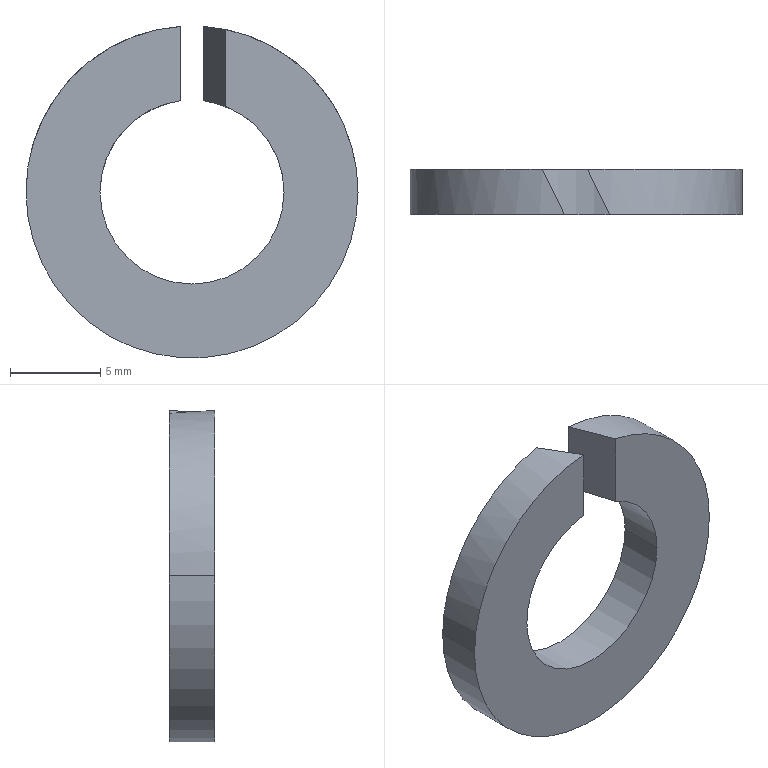Part | STEP file | ZZ24-M10-6 | 1 solid | 10 faces | box 18.4 x 2.5 x 18.378 mm | volume 434.673 mm3 | cylinder 6 | plane 4 | commonest cylinder face diameters 10.2 x3 18.4 x3
STEP:
#1=CARTESIAN_POINT('',(0.,0.,0.));
#2=DIRECTION('',(0.,0.,1.));
#3=DIRECTION('',(1.,0.,0.));
#4=AXIS2_PLACEMENT_3D('',#1,#2,#3);
#5=CARTESIAN_POINT('',(1.86,0.,4.749));
#6=VERTEX_POINT('',#5);
#7=CARTESIAN_POINT('',(0.6403,2.5,5.06));
#8=VERTEX_POINT('',#7);
#9=CARTESIAN_POINT('',(1.86,0.,4.749));
#10=CARTESIAN_POINT('',(1.467,0.8049,4.903));
#11=CARTESIAN_POINT('',(1.059,1.642,5.007));
#12=CARTESIAN_POINT('',(0.6403,2.5,5.06));
#13=(BOUNDED_CURVE()B_SPLINE_CURVE(3,(#9,#10,#11,#12),.UNSPECIFIED.,.F.,.F.)B_SPLINE_CURVE_WITH_KNOTS((4,4),(1.198,1.445),.PIECEWISE_BEZIER_KNOTS.)CURVE()GEOMETRIC_REPRESENTATION_ITEM()RATIONAL_B_SPLINE_CURVE((1.,0.9949,0.9949,1.))REPRESENTATION_ITEM(''));
#14=CARTESIAN_POINT('',(0.,2.5,0.));
#15=DIRECTION('',(0.,-1.,0.));
#16=DIRECTION('',(-1.,0.,0.001512));
#17=AXIS2_PLACEMENT_3D('',#14,#15,#16);
#18=CYLINDRICAL_SURFACE('',#17,5.1);
#19=CARTESIAN_POINT('',(4.341,2.5));
#20=CARTESIAN_POINT('',(4.344,2.464));
#21=CARTESIAN_POINT('',(4.352,2.391));
#22=CARTESIAN_POINT('',(4.363,2.281));
#23=CARTESIAN_POINT('',(4.374,2.17));
#24=CARTESIAN_POINT('',(4.386,2.059));
#25=CARTESIAN_POINT('',(4.397,1.948));
#26=CARTESIAN_POINT('',(4.408,1.836));
#27=CARTESIAN_POINT('',(4.419,1.723));
#28=CARTESIAN_POINT('',(4.431,1.61));
#29=CARTESIAN_POINT('',(4.442,1.497));
#30=CARTESIAN_POINT('',(4.453,1.384));
#31=CARTESIAN_POINT('',(4.464,1.27));
#32=CARTESIAN_POINT('',(4.476,1.156));
#33=CARTESIAN_POINT('',(4.487,1.041));
#34=CARTESIAN_POINT('',(4.498,0.9262));
#35=CARTESIAN_POINT('',(4.509,0.8111));
#36=CARTESIAN_POINT('',(4.521,0.6958));
#37=CARTESIAN_POINT('',(4.532,0.5802));
#38=CARTESIAN_POINT('',(4.543,0.4645));
#39=CARTESIAN_POINT('',(4.554,0.3486));
#40=CARTESIAN_POINT('',(4.566,0.2325));
#41=CARTESIAN_POINT('',(4.577,0.1163));
#42=CARTESIAN_POINT('',(4.584,0.03878));
#43=CARTESIAN_POINT('',(4.588,0.));
#44=B_SPLINE_CURVE_WITH_KNOTS('',3,(#19,#20,#21,#22,#23,#24,#25,#26,#27,#28,#29,#30,#31,#32,#33,#34,#35,#36,#37,#38,#39,#40,#41,#42,#43),.UNSPECIFIED.,.F.,.F.,(4,1,1,1,1,1,1,1,1,1,1,1,1,1,1,1,1,1,1,1,1,1,4),(1.198,1.209,1.22,1.231,1.243,1.254,1.265,1.276,1.287,1.299,1.31,1.321,1.332,1.344,1.355,1.366,1.377,1.389,1.4,1.411,1.422,1.434,1.445),.QUASI_UNIFORM_KNOTS.);
#45=(GEOMETRIC_REPRESENTATION_CONTEXT(2)PARAMETRIC_REPRESENTATION_CONTEXT()REPRESENTATION_CONTEXT('',''));
#46=DEFINITIONAL_REPRESENTATION('',(#44),#45);
#47=PCURVE('',#18,#46);
#48=CARTESIAN_POINT('',(1.86,0.,9.2));
#49=DIRECTION('',(-0.8988,-0.4384,0.));
#50=DIRECTION('',(0.4384,-0.8988,0.));
#51=AXIS2_PLACEMENT_3D('',#48,#49,#50);
#52=PLANE('',#51);
#53=CARTESIAN_POINT('',(0.,-4.451));
#54=CARTESIAN_POINT('',(-0.8955,-4.297));
#55=CARTESIAN_POINT('',(-1.827,-4.193));
#56=CARTESIAN_POINT('',(-2.782,-4.14));
#57=(BOUNDED_CURVE()B_SPLINE_CURVE(3,(#53,#54,#55,#56),.UNSPECIFIED.,.F.,.F.)B_SPLINE_CURVE_WITH_KNOTS((4,4),(1.198,1.445),.PIECEWISE_BEZIER_KNOTS.)CURVE()GEOMETRIC_REPRESENTATION_ITEM()RATIONAL_B_SPLINE_CURVE((1.,0.9949,0.9949,1.))REPRESENTATION_ITEM(''));
#58=(GEOMETRIC_REPRESENTATION_CONTEXT(2)PARAMETRIC_REPRESENTATION_CONTEXT()REPRESENTATION_CONTEXT('',''));
#59=DEFINITIONAL_REPRESENTATION('',(#57),#58);
#60=PCURVE('',#52,#59);
#61=SURFACE_CURVE('',#13,(#47,#60),.PCURVE_S1.);
#62=EDGE_CURVE('',#6,#8,#61,.T.);
#63=ORIENTED_EDGE('',*,*,#62,.F.);
#64=CARTESIAN_POINT('',(5.1,0.,-0.007712));
#65=VERTEX_POINT('',#64);
#66=CARTESIAN_POINT('',(0.,0.,0.));
#67=DIRECTION('',(0.,1.,0.));
#68=DIRECTION('',(1.,0.,-0.001512));
#69=AXIS2_PLACEMENT_3D('',#66,#67,#68);
#70=CIRCLE('',#69,5.1);
#71=CARTESIAN_POINT('',(9.425,2.5));
#72=DIRECTION('',(-1.,0.));
#73=VECTOR('',#72,1.);
#74=LINE('',#71,#73);
#75=(GEOMETRIC_REPRESENTATION_CONTEXT(2)PARAMETRIC_REPRESENTATION_CONTEXT()REPRESENTATION_CONTEXT('',''));
#76=DEFINITIONAL_REPRESENTATION('',(#74),#75);
#77=PCURVE('',#18,#76);
#78=CARTESIAN_POINT('',(0.,0.,0.));
#79=DIRECTION('',(0.,-1.,0.));
#80=DIRECTION('',(-1.,0.,0.001512));
#81=AXIS2_PLACEMENT_3D('',#78,#79,#80);
#82=PLANE('',#81);
#83=CARTESIAN_POINT('',(-5.1,0.));
#84=CARTESIAN_POINT('',(-5.1,8.833));
#85=CARTESIAN_POINT('',(2.55,4.417));
#86=CARTESIAN_POINT('',(10.2,0.));
#87=CARTESIAN_POINT('',(2.55,-4.417));
#88=CARTESIAN_POINT('',(-5.1,-8.833));
#89=CARTESIAN_POINT('',(-5.1,0.));
#90=(BOUNDED_CURVE()B_SPLINE_CURVE(2,(#83,#84,#85,#86,#87,#88,#89),.UNSPECIFIED.,.T.,.F.)B_SPLINE_CURVE_WITH_KNOTS((1,2,2,2,2,1),(-2.094,0.,2.094,4.189,6.283,8.378),.UNSPECIFIED.)CURVE()GEOMETRIC_REPRESENTATION_ITEM()RATIONAL_B_SPLINE_CURVE((1.,0.5,1.,0.5,1.,0.5,1.))REPRESENTATION_ITEM(''));
#91=(GEOMETRIC_REPRESENTATION_CONTEXT(2)PARAMETRIC_REPRESENTATION_CONTEXT()REPRESENTATION_CONTEXT('',''));
#92=DEFINITIONAL_REPRESENTATION('',(#90),#91);
#93=PCURVE('',#82,#92);
#94=SURFACE_CURVE('',#70,(#77,#93),.PCURVE_S1.);
#95=EDGE_CURVE('',#6,#65,#94,.T.);
#96=ORIENTED_EDGE('',*,*,#95,.T.);
#97=CARTESIAN_POINT('',(5.1,2.5,-0.007712));
#98=VERTEX_POINT('',#97);
#99=CARTESIAN_POINT('',(5.1,2.5,-0.007712));
#100=DIRECTION('',(0.,-1.,0.));
#101=VECTOR('',#100,1.);
#102=LINE('',#99,#101);
#103=CARTESIAN_POINT('',(3.142,0.));
#104=DIRECTION('',(0.,1.));
#105=VECTOR('',#104,1.);
#106=LINE('',#103,#105);
#107=(GEOMETRIC_REPRESENTATION_CONTEXT(2)PARAMETRIC_REPRESENTATION_CONTEXT()REPRESENTATION_CONTEXT('',''));
#108=DEFINITIONAL_REPRESENTATION('',(#106),#107);
#109=PCURVE('',#18,#108);
#110=CARTESIAN_POINT('',(0.,2.5,0.));
#111=DIRECTION('',(0.,-1.,0.));
#112=DIRECTION('',(-1.,0.,0.001512));
#113=AXIS2_PLACEMENT_3D('',#110,#111,#112);
#114=CYLINDRICAL_SURFACE('',#113,5.1);
#115=CARTESIAN_POINT('',(3.142,0.));
#116=DIRECTION('',(0.,1.));
#117=VECTOR('',#116,1.);
#118=LINE('',#115,#117);
#119=(GEOMETRIC_REPRESENTATION_CONTEXT(2)PARAMETRIC_REPRESENTATION_CONTEXT()REPRESENTATION_CONTEXT('',''));
#120=DEFINITIONAL_REPRESENTATION('',(#118),#119);
#121=PCURVE('',#114,#120);
#122=SURFACE_CURVE('',#102,(#109,#121),.PCURVE_S1.);
#123=EDGE_CURVE('',#98,#65,#122,.T.);
#124=ORIENTED_EDGE('',*,*,#123,.F.);
#125=CARTESIAN_POINT('',(0.,2.5,0.));
#126=DIRECTION('',(0.,-1.,0.));
#127=DIRECTION('',(-1.,0.,0.001512));
#128=AXIS2_PLACEMENT_3D('',#125,#126,#127);
#129=CIRCLE('',#128,5.1);
#130=CARTESIAN_POINT('',(0.,0.));
#131=DIRECTION('',(1.,0.));
#132=VECTOR('',#131,1.);
#133=LINE('',#130,#132);
#134=(GEOMETRIC_REPRESENTATION_CONTEXT(2)PARAMETRIC_REPRESENTATION_CONTEXT()REPRESENTATION_CONTEXT('',''));
#135=DEFINITIONAL_REPRESENTATION('',(#133),#134);
#136=PCURVE('',#18,#135);
#137=CARTESIAN_POINT('',(0.,2.5,0.));
#138=DIRECTION('',(0.,1.,0.));
#139=DIRECTION('',(1.,0.,-0.001512));
#140=AXIS2_PLACEMENT_3D('',#137,#138,#139);
#141=PLANE('',#140);
#142=CARTESIAN_POINT('',(-5.1,0.));
#143=CARTESIAN_POINT('',(-5.1,8.833));
#144=CARTESIAN_POINT('',(2.55,4.417));
#145=CARTESIAN_POINT('',(10.2,0.));
#146=CARTESIAN_POINT('',(2.55,-4.417));
#147=CARTESIAN_POINT('',(-5.1,-8.833));
#148=CARTESIAN_POINT('',(-5.1,0.));
#149=(BOUNDED_CURVE()B_SPLINE_CURVE(2,(#142,#143,#144,#145,#146,#147,#148),.UNSPECIFIED.,.T.,.F.)B_SPLINE_CURVE_WITH_KNOTS((1,2,2,2,2,1),(-2.094,0.,2.094,4.189,6.283,8.378),.UNSPECIFIED.)CURVE()GEOMETRIC_REPRESENTATION_ITEM()RATIONAL_B_SPLINE_CURVE((1.,0.5,1.,0.5,1.,0.5,1.))REPRESENTATION_ITEM(''));
#150=(GEOMETRIC_REPRESENTATION_CONTEXT(2)PARAMETRIC_REPRESENTATION_CONTEXT()REPRESENTATION_CONTEXT('',''));
#151=DEFINITIONAL_REPRESENTATION('',(#149),#150);
#152=PCURVE('',#141,#151);
#153=SURFACE_CURVE('',#129,(#136,#152),.PCURVE_S1.);
#154=EDGE_CURVE('',#98,#8,#153,.T.);
#155=ORIENTED_EDGE('',*,*,#154,.T.);
#156=EDGE_LOOP('',(#63,#96,#124,#155));
#157=FACE_BOUND('',#156,.F.);
#158=ADVANCED_FACE('',(#157),#18,.F.);
#159=CARTESIAN_POINT('',(-5.1,0.,0.007712));
#160=VERTEX_POINT('',#159);
#161=CARTESIAN_POINT('',(0.,0.,0.));
#162=DIRECTION('',(0.,1.,0.));
#163=DIRECTION('',(1.,0.,-0.001512));
#164=AXIS2_PLACEMENT_3D('',#161,#162,#163);
#165=CIRCLE('',#164,5.1);
#166=CARTESIAN_POINT('',(3.142,2.5));
#167=DIRECTION('',(-1.,0.));
#168=VECTOR('',#167,1.);
#169=LINE('',#166,#168);
#170=(GEOMETRIC_REPRESENTATION_CONTEXT(2)PARAMETRIC_REPRESENTATION_CONTEXT()REPRESENTATION_CONTEXT('',''));
#171=DEFINITIONAL_REPRESENTATION('',(#169),#170);
#172=PCURVE('',#114,#171);
#173=CARTESIAN_POINT('',(-5.1,0.));
#174=CARTESIAN_POINT('',(-5.1,8.833));
#175=CARTESIAN_POINT('',(2.55,4.417));
#176=CARTESIAN_POINT('',(10.2,0.));
#177=CARTESIAN_POINT('',(2.55,-4.417));
#178=CARTESIAN_POINT('',(-5.1,-8.833));
#179=CARTESIAN_POINT('',(-5.1,0.));
#180=(BOUNDED_CURVE()B_SPLINE_CURVE(2,(#173,#174,#175,#176,#177,#178,#179),.UNSPECIFIED.,.T.,.F.)B_SPLINE_CURVE_WITH_KNOTS((1,2,2,2,2,1),(-2.094,0.,2.094,4.189,6.283,8.378),.UNSPECIFIED.)CURVE()GEOMETRIC_REPRESENTATION_ITEM()RATIONAL_B_SPLINE_CURVE((1.,0.5,1.,0.5,1.,0.5,1.))REPRESENTATION_ITEM(''));
#181=(GEOMETRIC_REPRESENTATION_CONTEXT(2)PARAMETRIC_REPRESENTATION_CONTEXT()REPRESENTATION_CONTEXT('',''));
#182=DEFINITIONAL_REPRESENTATION('',(#180),#181);
#183=PCURVE('',#82,#182);
#184=SURFACE_CURVE('',#165,(#172,#183),.PCURVE_S1.);
#185=EDGE_CURVE('',#65,#160,#184,.T.);
#186=ORIENTED_EDGE('',*,*,#185,.T.);
#187=CARTESIAN_POINT('',(-5.1,2.5,0.007712));
#188=VERTEX_POINT('',#187);
#189=CARTESIAN_POINT('',(-5.1,2.5,0.007712));
#190=DIRECTION('',(0.,-1.,0.));
#191=VECTOR('',#190,1.);
#192=LINE('',#189,#191);
#193=CARTESIAN_POINT('',(0.,0.));
#194=DIRECTION('',(0.,1.));
#195=VECTOR('',#194,1.);
#196=LINE('',#193,#195);
#197=(GEOMETRIC_REPRESENTATION_CONTEXT(2)PARAMETRIC_REPRESENTATION_CONTEXT()REPRESENTATION_CONTEXT('',''));
#198=DEFINITIONAL_REPRESENTATION('',(#196),#197);
#199=PCURVE('',#114,#198);
#200=CARTESIAN_POINT('',(0.,2.5,0.));
#201=DIRECTION('',(0.,-1.,0.));
#202=DIRECTION('',(-1.,0.,0.001512));
#203=AXIS2_PLACEMENT_3D('',#200,#201,#202);
#204=CYLINDRICAL_SURFACE('',#203,5.1);
#205=CARTESIAN_POINT('',(6.283,0.));
#206=DIRECTION('',(0.,1.));
#207=VECTOR('',#206,1.);
#208=LINE('',#205,#207);
#209=(GEOMETRIC_REPRESENTATION_CONTEXT(2)PARAMETRIC_REPRESENTATION_CONTEXT()REPRESENTATION_CONTEXT('',''));
#210=DEFINITIONAL_REPRESENTATION('',(#208),#209);
#211=PCURVE('',#204,#210);
#212=SURFACE_CURVE('',#192,(#199,#211),.PCURVE_S1.);
#213=EDGE_CURVE('',#188,#160,#212,.T.);
#214=ORIENTED_EDGE('',*,*,#213,.F.);
#215=CARTESIAN_POINT('',(0.,2.5,0.));
#216=DIRECTION('',(0.,-1.,0.));
#217=DIRECTION('',(-1.,0.,0.001512));
#218=AXIS2_PLACEMENT_3D('',#215,#216,#217);
#219=CIRCLE('',#218,5.1);
#220=CARTESIAN_POINT('',(0.,0.));
#221=DIRECTION('',(1.,0.));
#222=VECTOR('',#221,1.);
#223=LINE('',#220,#222);
#224=(GEOMETRIC_REPRESENTATION_CONTEXT(2)PARAMETRIC_REPRESENTATION_CONTEXT()REPRESENTATION_CONTEXT('',''));
#225=DEFINITIONAL_REPRESENTATION('',(#223),#224);
#226=PCURVE('',#114,#225);
#227=CARTESIAN_POINT('',(-5.1,0.));
#228=CARTESIAN_POINT('',(-5.1,8.833));
#229=CARTESIAN_POINT('',(2.55,4.417));
#230=CARTESIAN_POINT('',(10.2,0.));
#231=CARTESIAN_POINT('',(2.55,-4.417));
#232=CARTESIAN_POINT('',(-5.1,-8.833));
#233=CARTESIAN_POINT('',(-5.1,0.));
#234=(BOUNDED_CURVE()B_SPLINE_CURVE(2,(#227,#228,#229,#230,#231,#232,#233),.UNSPECIFIED.,.T.,.F.)B_SPLINE_CURVE_WITH_KNOTS((1,2,2,2,2,1),(-2.094,0.,2.094,4.189,6.283,8.378),.UNSPECIFIED.)CURVE()GEOMETRIC_REPRESENTATION_ITEM()RATIONAL_B_SPLINE_CURVE((1.,0.5,1.,0.5,1.,0.5,1.))REPRESENTATION_ITEM(''));
#235=(GEOMETRIC_REPRESENTATION_CONTEXT(2)PARAMETRIC_REPRESENTATION_CONTEXT()REPRESENTATION_CONTEXT('',''));
#236=DEFINITIONAL_REPRESENTATION('',(#234),#235);
#237=PCURVE('',#141,#236);
#238=SURFACE_CURVE('',#219,(#226,#237),.PCURVE_S1.);
#239=EDGE_CURVE('',#188,#98,#238,.T.);
#240=ORIENTED_EDGE('',*,*,#239,.T.);
#241=ORIENTED_EDGE('',*,*,#123,.T.);
#242=EDGE_LOOP('',(#186,#214,#240,#241));
#243=FACE_BOUND('',#242,.F.);
#244=ADVANCED_FACE('',(#243),#114,.F.);
#245=CARTESIAN_POINT('',(-9.2,2.5,0.01391));
#246=VERTEX_POINT('',#245);
#247=CARTESIAN_POINT('',(9.2,2.5,-0.01391));
#248=VERTEX_POINT('',#247);
#249=CARTESIAN_POINT('',(0.,2.5,0.));
#250=DIRECTION('',(0.,-1.,0.));
#251=DIRECTION('',(-1.,0.,0.001512));
#252=AXIS2_PLACEMENT_3D('',#249,#250,#251);
#253=CIRCLE('',#252,9.2);
#254=CARTESIAN_POINT('',(0.,2.5,0.));
#255=DIRECTION('',(0.,-1.,0.));
#256=DIRECTION('',(-1.,0.,0.001512));
#257=AXIS2_PLACEMENT_3D('',#254,#255,#256);
#258=CYLINDRICAL_SURFACE('',#257,9.2);
#259=CARTESIAN_POINT('',(0.,0.));
#260=DIRECTION('',(1.,0.));
#261=VECTOR('',#260,1.);
#262=LINE('',#259,#261);
#263=(GEOMETRIC_REPRESENTATION_CONTEXT(2)PARAMETRIC_REPRESENTATION_CONTEXT()REPRESENTATION_CONTEXT('',''));
#264=DEFINITIONAL_REPRESENTATION('',(#262),#263);
#265=PCURVE('',#258,#264);
#266=CARTESIAN_POINT('',(-9.2,0.));
#267=CARTESIAN_POINT('',(-9.2,15.935));
#268=CARTESIAN_POINT('',(4.6,7.967));
#269=CARTESIAN_POINT('',(18.4,0.));
#270=CARTESIAN_POINT('',(4.6,-7.967));
#271=CARTESIAN_POINT('',(-9.2,-15.935));
#272=CARTESIAN_POINT('',(-9.2,0.));
#273=(BOUNDED_CURVE()B_SPLINE_CURVE(2,(#266,#267,#268,#269,#270,#271,#272),.UNSPECIFIED.,.T.,.F.)B_SPLINE_CURVE_WITH_KNOTS((1,2,2,2,2,1),(-2.094,0.,2.094,4.189,6.283,8.378),.UNSPECIFIED.)CURVE()GEOMETRIC_REPRESENTATION_ITEM()RATIONAL_B_SPLINE_CURVE((1.,0.5,1.,0.5,1.,0.5,1.))REPRESENTATION_ITEM(''));
#274=(GEOMETRIC_REPRESENTATION_CONTEXT(2)PARAMETRIC_REPRESENTATION_CONTEXT()REPRESENTATION_CONTEXT('',''));
#275=DEFINITIONAL_REPRESENTATION('',(#273),#274);
#276=PCURVE('',#141,#275);
#277=SURFACE_CURVE('',#253,(#265,#276),.PCURVE_S1.);
#278=EDGE_CURVE('',#246,#248,#277,.T.);
#279=ORIENTED_EDGE('',*,*,#278,.T.);
#280=CARTESIAN_POINT('',(9.2,0.,-0.01391));
#281=VERTEX_POINT('',#280);
#282=CARTESIAN_POINT('',(9.2,2.5,-0.01391));
#283=DIRECTION('',(0.,-1.,0.));
#284=VECTOR('',#283,1.);
#285=LINE('',#282,#284);
#286=CARTESIAN_POINT('',(3.142,0.));
#287=DIRECTION('',(0.,1.));
#288=VECTOR('',#287,1.);
#289=LINE('',#286,#288);
#290=(GEOMETRIC_REPRESENTATION_CONTEXT(2)PARAMETRIC_REPRESENTATION_CONTEXT()REPRESENTATION_CONTEXT('',''));
#291=DEFINITIONAL_REPRESENTATION('',(#289),#290);
#292=PCURVE('',#258,#291);
#293=CARTESIAN_POINT('',(0.,2.5,0.));
#294=DIRECTION('',(0.,-1.,0.));
#295=DIRECTION('',(-1.,0.,0.001512));
#296=AXIS2_PLACEMENT_3D('',#293,#294,#295);
#297=CYLINDRICAL_SURFACE('',#296,9.2);
#298=CARTESIAN_POINT('',(3.142,0.));
#299=DIRECTION('',(0.,1.));
#300=VECTOR('',#299,1.);
#301=LINE('',#298,#300);
#302=(GEOMETRIC_REPRESENTATION_CONTEXT(2)PARAMETRIC_REPRESENTATION_CONTEXT()REPRESENTATION_CONTEXT('',''));
#303=DEFINITIONAL_REPRESENTATION('',(#301),#302);
#304=PCURVE('',#297,#303);
#305=SURFACE_CURVE('',#285,(#292,#304),.PCURVE_S1.);
#306=EDGE_CURVE('',#248,#281,#305,.T.);
#307=ORIENTED_EDGE('',*,*,#306,.T.);
#308=CARTESIAN_POINT('',(-9.2,0.,0.01391));
#309=VERTEX_POINT('',#308);
#310=CARTESIAN_POINT('',(0.,0.,0.));
#311=DIRECTION('',(0.,1.,0.));
#312=DIRECTION('',(1.,0.,-0.001512));
#313=AXIS2_PLACEMENT_3D('',#310,#311,#312);
#314=CIRCLE('',#313,9.2);
#315=CARTESIAN_POINT('',(3.142,2.5));
#316=DIRECTION('',(-1.,0.));
#317=VECTOR('',#316,1.);
#318=LINE('',#315,#317);
#319=(GEOMETRIC_REPRESENTATION_CONTEXT(2)PARAMETRIC_REPRESENTATION_CONTEXT()REPRESENTATION_CONTEXT('',''));
#320=DEFINITIONAL_REPRESENTATION('',(#318),#319);
#321=PCURVE('',#258,#320);
#322=CARTESIAN_POINT('',(-9.2,0.));
#323=CARTESIAN_POINT('',(-9.2,15.935));
#324=CARTESIAN_POINT('',(4.6,7.967));
#325=CARTESIAN_POINT('',(18.4,0.));
#326=CARTESIAN_POINT('',(4.6,-7.967));
#327=CARTESIAN_POINT('',(-9.2,-15.935));
#328=CARTESIAN_POINT('',(-9.2,0.));
#329=(BOUNDED_CURVE()B_SPLINE_CURVE(2,(#322,#323,#324,#325,#326,#327,#328),.UNSPECIFIED.,.T.,.F.)B_SPLINE_CURVE_WITH_KNOTS((1,2,2,2,2,1),(-2.094,0.,2.094,4.189,6.283,8.378),.UNSPECIFIED.)CURVE()GEOMETRIC_REPRESENTATION_ITEM()RATIONAL_B_SPLINE_CURVE((1.,0.5,1.,0.5,1.,0.5,1.))REPRESENTATION_ITEM(''));
#330=(GEOMETRIC_REPRESENTATION_CONTEXT(2)PARAMETRIC_REPRESENTATION_CONTEXT()REPRESENTATION_CONTEXT('',''));
#331=DEFINITIONAL_REPRESENTATION('',(#329),#330);
#332=PCURVE('',#82,#331);
#333=SURFACE_CURVE('',#314,(#321,#332),.PCURVE_S1.);
#334=EDGE_CURVE('',#281,#309,#333,.T.);
#335=ORIENTED_EDGE('',*,*,#334,.T.);
#336=CARTESIAN_POINT('',(-9.2,2.5,0.01391));
#337=DIRECTION('',(0.,-1.,0.));
#338=VECTOR('',#337,1.);
#339=LINE('',#336,#338);
#340=CARTESIAN_POINT('',(0.,0.));
#341=DIRECTION('',(0.,1.));
#342=VECTOR('',#341,1.);
#343=LINE('',#340,#342);
#344=(GEOMETRIC_REPRESENTATION_CONTEXT(2)PARAMETRIC_REPRESENTATION_CONTEXT()REPRESENTATION_CONTEXT('',''));
#345=DEFINITIONAL_REPRESENTATION('',(#343),#344);
#346=PCURVE('',#258,#345);
#347=CARTESIAN_POINT('',(0.,2.5,0.));
#348=DIRECTION('',(0.,-1.,0.));
#349=DIRECTION('',(-1.,0.,0.001512));
#350=AXIS2_PLACEMENT_3D('',#347,#348,#349);
#351=CYLINDRICAL_SURFACE('',#350,9.2);
#352=CARTESIAN_POINT('',(6.283,0.));
#353=DIRECTION('',(0.,1.));
#354=VECTOR('',#353,1.);
#355=LINE('',#352,#354);
#356=(GEOMETRIC_REPRESENTATION_CONTEXT(2)PARAMETRIC_REPRESENTATION_CONTEXT()REPRESENTATION_CONTEXT('',''));
#357=DEFINITIONAL_REPRESENTATION('',(#355),#356);
#358=PCURVE('',#351,#357);
#359=SURFACE_CURVE('',#339,(#346,#358),.PCURVE_S1.);
#360=EDGE_CURVE('',#246,#309,#359,.T.);
#361=ORIENTED_EDGE('',*,*,#360,.F.);
#362=EDGE_LOOP('',(#279,#307,#335,#361));
#363=FACE_BOUND('',#362,.T.);
#364=ADVANCED_FACE('',(#363),#258,.T.);
#365=CARTESIAN_POINT('',(-1.86,2.5,9.01));
#366=VERTEX_POINT('',#365);
#367=CARTESIAN_POINT('',(0.,2.5,0.));
#368=DIRECTION('',(0.,-1.,0.));
#369=DIRECTION('',(-1.,0.,0.001512));
#370=AXIS2_PLACEMENT_3D('',#367,#368,#369);
#371=CIRCLE('',#370,9.2);
#372=CARTESIAN_POINT('',(0.,0.));
#373=DIRECTION('',(1.,0.));
#374=VECTOR('',#373,1.);
#375=LINE('',#372,#374);
#376=(GEOMETRIC_REPRESENTATION_CONTEXT(2)PARAMETRIC_REPRESENTATION_CONTEXT()REPRESENTATION_CONTEXT('',''));
#377=DEFINITIONAL_REPRESENTATION('',(#375),#376);
#378=PCURVE('',#351,#377);
#379=CARTESIAN_POINT('',(-9.2,0.));
#380=CARTESIAN_POINT('',(-9.2,15.935));
#381=CARTESIAN_POINT('',(4.6,7.967));
#382=CARTESIAN_POINT('',(18.4,0.));
#383=CARTESIAN_POINT('',(4.6,-7.967));
#384=CARTESIAN_POINT('',(-9.2,-15.935));
#385=CARTESIAN_POINT('',(-9.2,0.));
#386=(BOUNDED_CURVE()B_SPLINE_CURVE(2,(#379,#380,#381,#382,#383,#384,#385),.UNSPECIFIED.,.T.,.F.)B_SPLINE_CURVE_WITH_KNOTS((1,2,2,2,2,1),(-2.094,0.,2.094,4.189,6.283,8.378),.UNSPECIFIED.)CURVE()GEOMETRIC_REPRESENTATION_ITEM()RATIONAL_B_SPLINE_CURVE((1.,0.5,1.,0.5,1.,0.5,1.))REPRESENTATION_ITEM(''));
#387=(GEOMETRIC_REPRESENTATION_CONTEXT(2)PARAMETRIC_REPRESENTATION_CONTEXT()REPRESENTATION_CONTEXT('',''));
#388=DEFINITIONAL_REPRESENTATION('',(#386),#387);
#389=PCURVE('',#141,#388);
#390=SURFACE_CURVE('',#371,(#378,#389),.PCURVE_S1.);
#391=EDGE_CURVE('',#366,#246,#390,.T.);
#392=ORIENTED_EDGE('',*,*,#391,.T.);
#393=ORIENTED_EDGE('',*,*,#360,.T.);
#394=CARTESIAN_POINT('',(-0.6403,0.,9.178));
#395=VERTEX_POINT('',#394);
#396=CARTESIAN_POINT('',(0.,0.,0.));
#397=DIRECTION('',(0.,1.,0.));
#398=DIRECTION('',(1.,0.,-0.001512));
#399=AXIS2_PLACEMENT_3D('',#396,#397,#398);
#400=CIRCLE('',#399,9.2);
#401=CARTESIAN_POINT('',(9.425,2.5));
#402=DIRECTION('',(-1.,0.));
#403=VECTOR('',#402,1.);
#404=LINE('',#401,#403);
#405=(GEOMETRIC_REPRESENTATION_CONTEXT(2)PARAMETRIC_REPRESENTATION_CONTEXT()REPRESENTATION_CONTEXT('',''));
#406=DEFINITIONAL_REPRESENTATION('',(#404),#405);
#407=PCURVE('',#351,#406);
#408=CARTESIAN_POINT('',(-9.2,0.));
#409=CARTESIAN_POINT('',(-9.2,15.935));
#410=CARTESIAN_POINT('',(4.6,7.967));
#411=CARTESIAN_POINT('',(18.4,0.));
#412=CARTESIAN_POINT('',(4.6,-7.967));
#413=CARTESIAN_POINT('',(-9.2,-15.935));
#414=CARTESIAN_POINT('',(-9.2,0.));
#415=(BOUNDED_CURVE()B_SPLINE_CURVE(2,(#408,#409,#410,#411,#412,#413,#414),.UNSPECIFIED.,.T.,.F.)B_SPLINE_CURVE_WITH_KNOTS((1,2,2,2,2,1),(-2.094,0.,2.094,4.189,6.283,8.378),.UNSPECIFIED.)CURVE()GEOMETRIC_REPRESENTATION_ITEM()RATIONAL_B_SPLINE_CURVE((1.,0.5,1.,0.5,1.,0.5,1.))REPRESENTATION_ITEM(''));
#416=(GEOMETRIC_REPRESENTATION_CONTEXT(2)PARAMETRIC_REPRESENTATION_CONTEXT()REPRESENTATION_CONTEXT('',''));
#417=DEFINITIONAL_REPRESENTATION('',(#415),#416);
#418=PCURVE('',#82,#417);
#419=SURFACE_CURVE('',#400,(#407,#418),.PCURVE_S1.);
#420=EDGE_CURVE('',#309,#395,#419,.T.);
#421=ORIENTED_EDGE('',*,*,#420,.T.);
#422=CARTESIAN_POINT('',(-0.6403,0.,9.178));
#423=CARTESIAN_POINT('',(-1.05,0.8404,9.149));
#424=CARTESIAN_POINT('',(-1.457,1.675,9.093));
#425=CARTESIAN_POINT('',(-1.86,2.5,9.01));
#426=(BOUNDED_CURVE()B_SPLINE_CURVE(3,(#422,#423,#424,#425),.UNSPECIFIED.,.F.,.F.)B_SPLINE_CURVE_WITH_KNOTS((4,4),(1.64,1.774),.PIECEWISE_BEZIER_KNOTS.)CURVE()GEOMETRIC_REPRESENTATION_ITEM()RATIONAL_B_SPLINE_CURVE((1.,0.9985,0.9985,1.))REPRESENTATION_ITEM(''));
#427=CARTESIAN_POINT('',(4.784,2.5));
#428=CARTESIAN_POINT('',(4.786,2.462));
#429=CARTESIAN_POINT('',(4.79,2.386));
#430=CARTESIAN_POINT('',(4.796,2.271));
#431=CARTESIAN_POINT('',(4.802,2.157));
#432=CARTESIAN_POINT('',(4.808,2.043));
#433=CARTESIAN_POINT('',(4.814,1.928));
#434=CARTESIAN_POINT('',(4.82,1.814));
#435=CARTESIAN_POINT('',(4.826,1.7));
#436=CARTESIAN_POINT('',(4.832,1.586));
#437=CARTESIAN_POINT('',(4.838,1.472));
#438=CARTESIAN_POINT('',(4.844,1.358));
#439=CARTESIAN_POINT('',(4.851,1.244));
#440=CARTESIAN_POINT('',(4.857,1.131));
#441=CARTESIAN_POINT('',(4.863,1.017));
#442=CARTESIAN_POINT('',(4.869,0.9034));
#443=CARTESIAN_POINT('',(4.875,0.79));
#444=CARTESIAN_POINT('',(4.881,0.6767));
#445=CARTESIAN_POINT('',(4.887,0.5636));
#446=CARTESIAN_POINT('',(4.893,0.4506));
#447=CARTESIAN_POINT('',(4.899,0.3377));
#448=CARTESIAN_POINT('',(4.905,0.225));
#449=CARTESIAN_POINT('',(4.911,0.1124));
#450=CARTESIAN_POINT('',(4.915,0.03745));
#451=CARTESIAN_POINT('',(4.917,0.));
#452=B_SPLINE_CURVE_WITH_KNOTS('',3,(#427,#428,#429,#430,#431,#432,#433,#434,#435,#436,#437,#438,#439,#440,#441,#442,#443,#444,#445,#446,#447,#448,#449,#450,#451),.UNSPECIFIED.,.F.,.F.,(4,1,1,1,1,1,1,1,1,1,1,1,1,1,1,1,1,1,1,1,1,1,4),(1.64,1.647,1.653,1.659,1.665,1.671,1.677,1.683,1.689,1.695,1.701,1.707,1.713,1.72,1.726,1.732,1.738,1.744,1.75,1.756,1.762,1.768,1.774),.QUASI_UNIFORM_KNOTS.);
#453=(GEOMETRIC_REPRESENTATION_CONTEXT(2)PARAMETRIC_REPRESENTATION_CONTEXT()REPRESENTATION_CONTEXT('',''));
#454=DEFINITIONAL_REPRESENTATION('',(#452),#453);
#455=PCURVE('',#351,#454);
#456=CARTESIAN_POINT('',(-1.86,2.5,9.2));
#457=DIRECTION('',(0.8988,0.4384,0.));
#458=DIRECTION('',(-0.4384,0.8988,0.));
#459=AXIS2_PLACEMENT_3D('',#456,#457,#458);
#460=PLANE('',#459);
#461=CARTESIAN_POINT('',(-2.782,-0.02231));
#462=CARTESIAN_POINT('',(-1.846,-0.05091));
#463=CARTESIAN_POINT('',(-0.9179,-0.1069));
#464=CARTESIAN_POINT('',(0.,-0.1899));
#465=(BOUNDED_CURVE()B_SPLINE_CURVE(3,(#461,#462,#463,#464),.UNSPECIFIED.,.F.,.F.)B_SPLINE_CURVE_WITH_KNOTS((4,4),(1.64,1.774),.PIECEWISE_BEZIER_KNOTS.)CURVE()GEOMETRIC_REPRESENTATION_ITEM()RATIONAL_B_SPLINE_CURVE((1.,0.9985,0.9985,1.))REPRESENTATION_ITEM(''));
#466=(GEOMETRIC_REPRESENTATION_CONTEXT(2)PARAMETRIC_REPRESENTATION_CONTEXT()REPRESENTATION_CONTEXT('',''));
#467=DEFINITIONAL_REPRESENTATION('',(#465),#466);
#468=PCURVE('',#460,#467);
#469=SURFACE_CURVE('',#426,(#455,#468),.PCURVE_S1.);
#470=EDGE_CURVE('',#395,#366,#469,.T.);
#471=ORIENTED_EDGE('',*,*,#470,.T.);
#472=EDGE_LOOP('',(#392,#393,#421,#471));
#473=FACE_BOUND('',#472,.T.);
#474=ADVANCED_FACE('',(#473),#351,.T.);
#475=CARTESIAN_POINT('',(-0.6403,0.,5.06));
#476=VERTEX_POINT('',#475);
#477=CARTESIAN_POINT('',(-0.6403,0.,9.2));
#478=DIRECTION('',(0.,0.,-1.));
#479=VECTOR('',#478,1.);
#480=LINE('',#477,#479);
#481=CARTESIAN_POINT('',(0.6542,-9.199));
#482=DIRECTION('',(-0.001512,1.));
#483=VECTOR('',#482,1.);
#484=LINE('',#481,#483);
#485=(GEOMETRIC_REPRESENTATION_CONTEXT(2)PARAMETRIC_REPRESENTATION_CONTEXT()REPRESENTATION_CONTEXT('',''));
#486=DEFINITIONAL_REPRESENTATION('',(#484),#485);
#487=PCURVE('',#82,#486);
#488=CARTESIAN_POINT('',(-2.782,0.));
#489=DIRECTION('',(0.,-1.));
#490=VECTOR('',#489,1.);
#491=LINE('',#488,#490);
#492=(GEOMETRIC_REPRESENTATION_CONTEXT(2)PARAMETRIC_REPRESENTATION_CONTEXT()REPRESENTATION_CONTEXT('',''));
#493=DEFINITIONAL_REPRESENTATION('',(#491),#492);
#494=PCURVE('',#460,#493);
#495=SURFACE_CURVE('',#480,(#487,#494),.PCURVE_S1.);
#496=EDGE_CURVE('',#395,#476,#495,.T.);
#497=ORIENTED_EDGE('',*,*,#496,.F.);
#498=ORIENTED_EDGE('',*,*,#420,.F.);
#499=ORIENTED_EDGE('',*,*,#334,.F.);
#500=CARTESIAN_POINT('',(1.86,0.,9.01));
#501=VERTEX_POINT('',#500);
#502=CARTESIAN_POINT('',(0.,0.,0.));
#503=DIRECTION('',(0.,1.,0.));
#504=DIRECTION('',(1.,0.,-0.001512));
#505=AXIS2_PLACEMENT_3D('',#502,#503,#504);
#506=CIRCLE('',#505,9.2);
#507=CARTESIAN_POINT('',(-9.2,0.));
#508=CARTESIAN_POINT('',(-9.2,15.935));
#509=CARTESIAN_POINT('',(4.6,7.967));
#510=CARTESIAN_POINT('',(18.4,0.));
#511=CARTESIAN_POINT('',(4.6,-7.967));
#512=CARTESIAN_POINT('',(-9.2,-15.935));
#513=CARTESIAN_POINT('',(-9.2,0.));
#514=(BOUNDED_CURVE()B_SPLINE_CURVE(2,(#507,#508,#509,#510,#511,#512,#513),.UNSPECIFIED.,.T.,.F.)B_SPLINE_CURVE_WITH_KNOTS((1,2,2,2,2,1),(-2.094,0.,2.094,4.189,6.283,8.378),.UNSPECIFIED.)CURVE()GEOMETRIC_REPRESENTATION_ITEM()RATIONAL_B_SPLINE_CURVE((1.,0.5,1.,0.5,1.,0.5,1.))REPRESENTATION_ITEM(''));
#515=(GEOMETRIC_REPRESENTATION_CONTEXT(2)PARAMETRIC_REPRESENTATION_CONTEXT()REPRESENTATION_CONTEXT('',''));
#516=DEFINITIONAL_REPRESENTATION('',(#514),#515);
#517=PCURVE('',#82,#516);
#518=CARTESIAN_POINT('',(9.425,2.5));
#519=DIRECTION('',(-1.,0.));
#520=VECTOR('',#519,1.);
#521=LINE('',#518,#520);
#522=(GEOMETRIC_REPRESENTATION_CONTEXT(2)PARAMETRIC_REPRESENTATION_CONTEXT()REPRESENTATION_CONTEXT('',''));
#523=DEFINITIONAL_REPRESENTATION('',(#521),#522);
#524=PCURVE('',#297,#523);
#525=SURFACE_CURVE('',#506,(#517,#524),.PCURVE_S1.);
#526=EDGE_CURVE('',#501,#281,#525,.T.);
#527=ORIENTED_EDGE('',*,*,#526,.F.);
#528=CARTESIAN_POINT('',(1.86,0.,9.2));
#529=DIRECTION('',(0.,0.,-1.));
#530=VECTOR('',#529,1.);
#531=LINE('',#528,#530);
#532=CARTESIAN_POINT('',(-1.846,-9.203));
#533=DIRECTION('',(-0.001512,1.));
#534=VECTOR('',#533,1.);
#535=LINE('',#532,#534);
#536=(GEOMETRIC_REPRESENTATION_CONTEXT(2)PARAMETRIC_REPRESENTATION_CONTEXT()REPRESENTATION_CONTEXT('',''));
#537=DEFINITIONAL_REPRESENTATION('',(#535),#536);
#538=PCURVE('',#82,#537);
#539=CARTESIAN_POINT('',(0.,0.));
#540=DIRECTION('',(0.,-1.));
#541=VECTOR('',#540,1.);
#542=LINE('',#539,#541);
#543=(GEOMETRIC_REPRESENTATION_CONTEXT(2)PARAMETRIC_REPRESENTATION_CONTEXT()REPRESENTATION_CONTEXT('',''));
#544=DEFINITIONAL_REPRESENTATION('',(#542),#543);
#545=PCURVE('',#52,#544);
#546=SURFACE_CURVE('',#531,(#538,#545),.PCURVE_S1.);
#547=EDGE_CURVE('',#501,#6,#546,.T.);
#548=ORIENTED_EDGE('',*,*,#547,.T.);
#549=ORIENTED_EDGE('',*,*,#95,.T.);
#550=ORIENTED_EDGE('',*,*,#185,.T.);
#551=CARTESIAN_POINT('',(0.,0.,0.));
#552=DIRECTION('',(0.,1.,0.));
#553=DIRECTION('',(1.,0.,-0.001512));
#554=AXIS2_PLACEMENT_3D('',#551,#552,#553);
#555=CIRCLE('',#554,5.1);
#556=CARTESIAN_POINT('',(-5.1,0.));
#557=CARTESIAN_POINT('',(-5.1,8.833));
#558=CARTESIAN_POINT('',(2.55,4.417));
#559=CARTESIAN_POINT('',(10.2,0.));
#560=CARTESIAN_POINT('',(2.55,-4.417));
#561=CARTESIAN_POINT('',(-5.1,-8.833));
#562=CARTESIAN_POINT('',(-5.1,0.));
#563=(BOUNDED_CURVE()B_SPLINE_CURVE(2,(#556,#557,#558,#559,#560,#561,#562),.UNSPECIFIED.,.T.,.F.)B_SPLINE_CURVE_WITH_KNOTS((1,2,2,2,2,1),(-2.094,0.,2.094,4.189,6.283,8.378),.UNSPECIFIED.)CURVE()GEOMETRIC_REPRESENTATION_ITEM()RATIONAL_B_SPLINE_CURVE((1.,0.5,1.,0.5,1.,0.5,1.))REPRESENTATION_ITEM(''));
#564=(GEOMETRIC_REPRESENTATION_CONTEXT(2)PARAMETRIC_REPRESENTATION_CONTEXT()REPRESENTATION_CONTEXT('',''));
#565=DEFINITIONAL_REPRESENTATION('',(#563),#564);
#566=PCURVE('',#82,#565);
#567=CARTESIAN_POINT('',(9.425,2.5));
#568=DIRECTION('',(-1.,0.));
#569=VECTOR('',#568,1.);
#570=LINE('',#567,#569);
#571=(GEOMETRIC_REPRESENTATION_CONTEXT(2)PARAMETRIC_REPRESENTATION_CONTEXT()REPRESENTATION_CONTEXT('',''));
#572=DEFINITIONAL_REPRESENTATION('',(#570),#571);
#573=PCURVE('',#204,#572);
#574=SURFACE_CURVE('',#555,(#566,#573),.PCURVE_S1.);
#575=EDGE_CURVE('',#160,#476,#574,.T.);
#576=ORIENTED_EDGE('',*,*,#575,.T.);
#577=EDGE_LOOP('',(#497,#498,#499,#527,#548,#549,#550,#576));
#578=FACE_BOUND('',#577,.T.);
#579=ADVANCED_FACE('',(#578),#82,.T.);
#580=CARTESIAN_POINT('',(0.6403,2.5,9.178));
#581=VERTEX_POINT('',#580);
#582=CARTESIAN_POINT('',(0.6403,2.5,9.2));
#583=DIRECTION('',(0.,0.,-1.));
#584=VECTOR('',#583,1.);
#585=LINE('',#582,#584);
#586=CARTESIAN_POINT('',(0.6264,-9.201));
#587=DIRECTION('',(0.001512,1.));
#588=VECTOR('',#587,1.);
#589=LINE('',#586,#588);
#590=(GEOMETRIC_REPRESENTATION_CONTEXT(2)PARAMETRIC_REPRESENTATION_CONTEXT()REPRESENTATION_CONTEXT('',''));
#591=DEFINITIONAL_REPRESENTATION('',(#589),#590);
#592=PCURVE('',#141,#591);
#593=CARTESIAN_POINT('',(-2.782,0.));
#594=DIRECTION('',(0.,-1.));
#595=VECTOR('',#594,1.);
#596=LINE('',#593,#595);
#597=(GEOMETRIC_REPRESENTATION_CONTEXT(2)PARAMETRIC_REPRESENTATION_CONTEXT()REPRESENTATION_CONTEXT('',''));
#598=DEFINITIONAL_REPRESENTATION('',(#596),#597);
#599=PCURVE('',#52,#598);
#600=SURFACE_CURVE('',#585,(#592,#599),.PCURVE_S1.);
#601=EDGE_CURVE('',#581,#8,#600,.T.);
#602=ORIENTED_EDGE('',*,*,#601,.F.);
#603=CARTESIAN_POINT('',(0.,2.5,0.));
#604=DIRECTION('',(0.,-1.,0.));
#605=DIRECTION('',(-1.,0.,0.001512));
#606=AXIS2_PLACEMENT_3D('',#603,#604,#605);
#607=CIRCLE('',#606,9.2);
#608=CARTESIAN_POINT('',(-9.2,0.));
#609=CARTESIAN_POINT('',(-9.2,15.935));
#610=CARTESIAN_POINT('',(4.6,7.967));
#611=CARTESIAN_POINT('',(18.4,0.));
#612=CARTESIAN_POINT('',(4.6,-7.967));
#613=CARTESIAN_POINT('',(-9.2,-15.935));
#614=CARTESIAN_POINT('',(-9.2,0.));
#615=(BOUNDED_CURVE()B_SPLINE_CURVE(2,(#608,#609,#610,#611,#612,#613,#614),.UNSPECIFIED.,.T.,.F.)B_SPLINE_CURVE_WITH_KNOTS((1,2,2,2,2,1),(-2.094,0.,2.094,4.189,6.283,8.378),.UNSPECIFIED.)CURVE()GEOMETRIC_REPRESENTATION_ITEM()RATIONAL_B_SPLINE_CURVE((1.,0.5,1.,0.5,1.,0.5,1.))REPRESENTATION_ITEM(''));
#616=(GEOMETRIC_REPRESENTATION_CONTEXT(2)PARAMETRIC_REPRESENTATION_CONTEXT()REPRESENTATION_CONTEXT('',''));
#617=DEFINITIONAL_REPRESENTATION('',(#615),#616);
#618=PCURVE('',#141,#617);
#619=CARTESIAN_POINT('',(0.,0.));
#620=DIRECTION('',(1.,0.));
#621=VECTOR('',#620,1.);
#622=LINE('',#619,#621);
#623=(GEOMETRIC_REPRESENTATION_CONTEXT(2)PARAMETRIC_REPRESENTATION_CONTEXT()REPRESENTATION_CONTEXT('',''));
#624=DEFINITIONAL_REPRESENTATION('',(#622),#623);
#625=PCURVE('',#297,#624);
#626=SURFACE_CURVE('',#607,(#618,#625),.PCURVE_S1.);
#627=EDGE_CURVE('',#248,#581,#626,.T.);
#628=ORIENTED_EDGE('',*,*,#627,.F.);
#629=ORIENTED_EDGE('',*,*,#278,.F.);
#630=ORIENTED_EDGE('',*,*,#391,.F.);
#631=CARTESIAN_POINT('',(-1.86,2.5,4.749));
#632=VERTEX_POINT('',#631);
#633=CARTESIAN_POINT('',(-1.86,2.5,9.2));
#634=DIRECTION('',(0.,0.,-1.));
#635=VECTOR('',#634,1.);
#636=LINE('',#633,#635);
#637=CARTESIAN_POINT('',(-1.874,-9.197));
#638=DIRECTION('',(0.001512,1.));
#639=VECTOR('',#638,1.);
#640=LINE('',#637,#639);
#641=(GEOMETRIC_REPRESENTATION_CONTEXT(2)PARAMETRIC_REPRESENTATION_CONTEXT()REPRESENTATION_CONTEXT('',''));
#642=DEFINITIONAL_REPRESENTATION('',(#640),#641);
#643=PCURVE('',#141,#642);
#644=CARTESIAN_POINT('',(0.,0.));
#645=DIRECTION('',(0.,-1.));
#646=VECTOR('',#645,1.);
#647=LINE('',#644,#646);
#648=(GEOMETRIC_REPRESENTATION_CONTEXT(2)PARAMETRIC_REPRESENTATION_CONTEXT()REPRESENTATION_CONTEXT('',''));
#649=DEFINITIONAL_REPRESENTATION('',(#647),#648);
#650=PCURVE('',#460,#649);
#651=SURFACE_CURVE('',#636,(#643,#650),.PCURVE_S1.);
#652=EDGE_CURVE('',#366,#632,#651,.T.);
#653=ORIENTED_EDGE('',*,*,#652,.T.);
#654=CARTESIAN_POINT('',(0.,2.5,0.));
#655=DIRECTION('',(0.,-1.,0.));
#656=DIRECTION('',(-1.,0.,0.001512));
#657=AXIS2_PLACEMENT_3D('',#654,#655,#656);
#658=CIRCLE('',#657,5.1);
#659=CARTESIAN_POINT('',(-5.1,0.));
#660=CARTESIAN_POINT('',(-5.1,8.833));
#661=CARTESIAN_POINT('',(2.55,4.417));
#662=CARTESIAN_POINT('',(10.2,0.));
#663=CARTESIAN_POINT('',(2.55,-4.417));
#664=CARTESIAN_POINT('',(-5.1,-8.833));
#665=CARTESIAN_POINT('',(-5.1,0.));
#666=(BOUNDED_CURVE()B_SPLINE_CURVE(2,(#659,#660,#661,#662,#663,#664,#665),.UNSPECIFIED.,.T.,.F.)B_SPLINE_CURVE_WITH_KNOTS((1,2,2,2,2,1),(-2.094,0.,2.094,4.189,6.283,8.378),.UNSPECIFIED.)CURVE()GEOMETRIC_REPRESENTATION_ITEM()RATIONAL_B_SPLINE_CURVE((1.,0.5,1.,0.5,1.,0.5,1.))REPRESENTATION_ITEM(''));
#667=(GEOMETRIC_REPRESENTATION_CONTEXT(2)PARAMETRIC_REPRESENTATION_CONTEXT()REPRESENTATION_CONTEXT('',''));
#668=DEFINITIONAL_REPRESENTATION('',(#666),#667);
#669=PCURVE('',#141,#668);
#670=CARTESIAN_POINT('',(0.,0.));
#671=DIRECTION('',(1.,0.));
#672=VECTOR('',#671,1.);
#673=LINE('',#670,#672);
#674=(GEOMETRIC_REPRESENTATION_CONTEXT(2)PARAMETRIC_REPRESENTATION_CONTEXT()REPRESENTATION_CONTEXT('',''));
#675=DEFINITIONAL_REPRESENTATION('',(#673),#674);
#676=PCURVE('',#204,#675);
#677=SURFACE_CURVE('',#658,(#669,#676),.PCURVE_S1.);
#678=EDGE_CURVE('',#632,#188,#677,.T.);
#679=ORIENTED_EDGE('',*,*,#678,.T.);
#680=ORIENTED_EDGE('',*,*,#239,.T.);
#681=ORIENTED_EDGE('',*,*,#154,.T.);
#682=EDGE_LOOP('',(#602,#628,#629,#630,#653,#679,#680,#681));
#683=FACE_BOUND('',#682,.T.);
#684=ADVANCED_FACE('',(#683),#141,.T.);
#685=ORIENTED_EDGE('',*,*,#306,.F.);
#686=ORIENTED_EDGE('',*,*,#627,.T.);
#687=CARTESIAN_POINT('',(0.6403,2.5,9.178));
#688=CARTESIAN_POINT('',(1.05,1.66,9.149));
#689=CARTESIAN_POINT('',(1.457,0.825,9.093));
#690=CARTESIAN_POINT('',(1.86,0.,9.01));
#691=(BOUNDED_CURVE()B_SPLINE_CURVE(3,(#687,#688,#689,#690),.UNSPECIFIED.,.F.,.F.)B_SPLINE_CURVE_WITH_KNOTS((4,4),(4.782,4.916),.PIECEWISE_BEZIER_KNOTS.)CURVE()GEOMETRIC_REPRESENTATION_ITEM()RATIONAL_B_SPLINE_CURVE((1.,0.9985,0.9985,1.))REPRESENTATION_ITEM(''));
#692=CARTESIAN_POINT('',(4.644,0.));
#693=CARTESIAN_POINT('',(4.642,0.03814));
#694=CARTESIAN_POINT('',(4.638,0.1144));
#695=CARTESIAN_POINT('',(4.632,0.2288));
#696=CARTESIAN_POINT('',(4.626,0.3431));
#697=CARTESIAN_POINT('',(4.62,0.4574));
#698=CARTESIAN_POINT('',(4.614,0.5717));
#699=CARTESIAN_POINT('',(4.608,0.6859));
#700=CARTESIAN_POINT('',(4.602,0.8));
#701=CARTESIAN_POINT('',(4.596,0.9141));
#702=CARTESIAN_POINT('',(4.589,1.028));
#703=CARTESIAN_POINT('',(4.583,1.142));
#704=CARTESIAN_POINT('',(4.577,1.256));
#705=CARTESIAN_POINT('',(4.571,1.369));
#706=CARTESIAN_POINT('',(4.565,1.483));
#707=CARTESIAN_POINT('',(4.559,1.597));
#708=CARTESIAN_POINT('',(4.553,1.71));
#709=CARTESIAN_POINT('',(4.547,1.823));
#710=CARTESIAN_POINT('',(4.541,1.936));
#711=CARTESIAN_POINT('',(4.535,2.049));
#712=CARTESIAN_POINT('',(4.529,2.162));
#713=CARTESIAN_POINT('',(4.523,2.275));
#714=CARTESIAN_POINT('',(4.516,2.388));
#715=CARTESIAN_POINT('',(4.512,2.463));
#716=CARTESIAN_POINT('',(4.51,2.5));
#717=B_SPLINE_CURVE_WITH_KNOTS('',3,(#692,#693,#694,#695,#696,#697,#698,#699,#700,#701,#702,#703,#704,#705,#706,#707,#708,#709,#710,#711,#712,#713,#714,#715,#716),.UNSPECIFIED.,.F.,.F.,(4,1,1,1,1,1,1,1,1,1,1,1,1,1,1,1,1,1,1,1,1,1,4),(4.782,4.788,4.794,4.8,4.806,4.812,4.819,4.825,4.831,4.837,4.843,4.849,4.855,4.861,4.867,4.873,4.879,4.886,4.892,4.898,4.904,4.91,4.916),.QUASI_UNIFORM_KNOTS.);
#718=(GEOMETRIC_REPRESENTATION_CONTEXT(2)PARAMETRIC_REPRESENTATION_CONTEXT()REPRESENTATION_CONTEXT('',''));
#719=DEFINITIONAL_REPRESENTATION('',(#717),#718);
#720=PCURVE('',#297,#719);
#721=CARTESIAN_POINT('',(-2.782,-0.02231));
#722=CARTESIAN_POINT('',(-1.846,-0.05091));
#723=CARTESIAN_POINT('',(-0.9179,-0.1069));
#724=CARTESIAN_POINT('',(0.,-0.1899));
#725=(BOUNDED_CURVE()B_SPLINE_CURVE(3,(#721,#722,#723,#724),.UNSPECIFIED.,.F.,.F.)B_SPLINE_CURVE_WITH_KNOTS((4,4),(4.782,4.916),.PIECEWISE_BEZIER_KNOTS.)CURVE()GEOMETRIC_REPRESENTATION_ITEM()RATIONAL_B_SPLINE_CURVE((1.,0.9985,0.9985,1.))REPRESENTATION_ITEM(''));
#726=(GEOMETRIC_REPRESENTATION_CONTEXT(2)PARAMETRIC_REPRESENTATION_CONTEXT()REPRESENTATION_CONTEXT('',''));
#727=DEFINITIONAL_REPRESENTATION('',(#725),#726);
#728=PCURVE('',#52,#727);
#729=SURFACE_CURVE('',#691,(#720,#728),.PCURVE_S1.);
#730=EDGE_CURVE('',#581,#501,#729,.T.);
#731=ORIENTED_EDGE('',*,*,#730,.T.);
#732=ORIENTED_EDGE('',*,*,#526,.T.);
#733=EDGE_LOOP('',(#685,#686,#731,#732));
#734=FACE_BOUND('',#733,.T.);
#735=ADVANCED_FACE('',(#734),#297,.T.);
#736=ORIENTED_EDGE('',*,*,#601,.T.);
#737=ORIENTED_EDGE('',*,*,#62,.F.);
#738=ORIENTED_EDGE('',*,*,#547,.F.);
#739=ORIENTED_EDGE('',*,*,#730,.F.);
#740=EDGE_LOOP('',(#736,#737,#738,#739));
#741=FACE_BOUND('',#740,.T.);
#742=ADVANCED_FACE('',(#741),#52,.T.);
#743=ORIENTED_EDGE('',*,*,#496,.T.);
#744=CARTESIAN_POINT('',(-1.86,2.5,4.749));
#745=CARTESIAN_POINT('',(-1.467,1.695,4.903));
#746=CARTESIAN_POINT('',(-1.059,0.8575,5.007));
#747=CARTESIAN_POINT('',(-0.6403,0.,5.06));
#748=(BOUNDED_CURVE()B_SPLINE_CURVE(3,(#744,#745,#746,#747),.UNSPECIFIED.,.F.,.F.)B_SPLINE_CURVE_WITH_KNOTS((4,4),(4.339,4.587),.PIECEWISE_BEZIER_KNOTS.)CURVE()GEOMETRIC_REPRESENTATION_ITEM()RATIONAL_B_SPLINE_CURVE((1.,0.9949,0.9949,1.))REPRESENTATION_ITEM(''));
#749=CARTESIAN_POINT('',(0.,-4.451));
#750=CARTESIAN_POINT('',(-0.8955,-4.297));
#751=CARTESIAN_POINT('',(-1.827,-4.193));
#752=CARTESIAN_POINT('',(-2.782,-4.14));
#753=(BOUNDED_CURVE()B_SPLINE_CURVE(3,(#749,#750,#751,#752),.UNSPECIFIED.,.F.,.F.)B_SPLINE_CURVE_WITH_KNOTS((4,4),(4.339,4.587),.PIECEWISE_BEZIER_KNOTS.)CURVE()GEOMETRIC_REPRESENTATION_ITEM()RATIONAL_B_SPLINE_CURVE((1.,0.9949,0.9949,1.))REPRESENTATION_ITEM(''));
#754=(GEOMETRIC_REPRESENTATION_CONTEXT(2)PARAMETRIC_REPRESENTATION_CONTEXT()REPRESENTATION_CONTEXT('',''));
#755=DEFINITIONAL_REPRESENTATION('',(#753),#754);
#756=PCURVE('',#460,#755);
#757=CARTESIAN_POINT('',(5.087,0.));
#758=CARTESIAN_POINT('',(5.083,0.0364));
#759=CARTESIAN_POINT('',(5.076,0.1094));
#760=CARTESIAN_POINT('',(5.065,0.2194));
#761=CARTESIAN_POINT('',(5.053,0.3299));
#762=CARTESIAN_POINT('',(5.042,0.4409));
#763=CARTESIAN_POINT('',(5.031,0.5524));
#764=CARTESIAN_POINT('',(5.02,0.6644));
#765=CARTESIAN_POINT('',(5.008,0.7768));
#766=CARTESIAN_POINT('',(4.997,0.8896));
#767=CARTESIAN_POINT('',(4.986,1.003));
#768=CARTESIAN_POINT('',(4.975,1.116));
#769=CARTESIAN_POINT('',(4.963,1.23));
#770=CARTESIAN_POINT('',(4.952,1.344));
#771=CARTESIAN_POINT('',(4.941,1.459));
#772=CARTESIAN_POINT('',(4.93,1.574));
#773=CARTESIAN_POINT('',(4.918,1.689));
#774=CARTESIAN_POINT('',(4.907,1.804));
#775=CARTESIAN_POINT('',(4.896,1.92));
#776=CARTESIAN_POINT('',(4.885,2.036));
#777=CARTESIAN_POINT('',(4.873,2.151));
#778=CARTESIAN_POINT('',(4.862,2.267));
#779=CARTESIAN_POINT('',(4.851,2.384));
#780=CARTESIAN_POINT('',(4.844,2.461));
#781=CARTESIAN_POINT('',(4.84,2.5));
#782=B_SPLINE_CURVE_WITH_KNOTS('',3,(#757,#758,#759,#760,#761,#762,#763,#764,#765,#766,#767,#768,#769,#770,#771,#772,#773,#774,#775,#776,#777,#778,#779,#780,#781),.UNSPECIFIED.,.F.,.F.,(4,1,1,1,1,1,1,1,1,1,1,1,1,1,1,1,1,1,1,1,1,1,4),(4.339,4.35,4.362,4.373,4.384,4.395,4.407,4.418,4.429,4.44,4.452,4.463,4.474,4.485,4.497,4.508,4.519,4.53,4.542,4.553,4.564,4.575,4.587),.QUASI_UNIFORM_KNOTS.);
#783=(GEOMETRIC_REPRESENTATION_CONTEXT(2)PARAMETRIC_REPRESENTATION_CONTEXT()REPRESENTATION_CONTEXT('',''));
#784=DEFINITIONAL_REPRESENTATION('',(#782),#783);
#785=PCURVE('',#204,#784);
#786=SURFACE_CURVE('',#748,(#756,#785),.PCURVE_S1.);
#787=EDGE_CURVE('',#632,#476,#786,.T.);
#788=ORIENTED_EDGE('',*,*,#787,.F.);
#789=ORIENTED_EDGE('',*,*,#652,.F.);
#790=ORIENTED_EDGE('',*,*,#470,.F.);
#791=EDGE_LOOP('',(#743,#788,#789,#790));
#792=FACE_BOUND('',#791,.T.);
#793=ADVANCED_FACE('',(#792),#460,.T.);
#794=ORIENTED_EDGE('',*,*,#575,.T.);
#795=ORIENTED_EDGE('',*,*,#787,.F.);
#796=ORIENTED_EDGE('',*,*,#678,.T.);
#797=ORIENTED_EDGE('',*,*,#213,.T.);
#798=EDGE_LOOP('',(#794,#795,#796,#797));
#799=FACE_BOUND('',#798,.F.);
#800=ADVANCED_FACE('',(#799),#204,.F.);
#801=CLOSED_SHELL('',(#158,#244,#364,#474,#579,#684,#735,#742,#793,#800));
#802=MANIFOLD_SOLID_BREP('',#801);
#803=(LENGTH_UNIT()NAMED_UNIT(*)SI_UNIT(.MILLI.,.METRE.));
#804=UNCERTAINTY_MEASURE_WITH_UNIT(LENGTH_MEASURE(0.0000001),#803,'','');
#805=(NAMED_UNIT(*)PLANE_ANGLE_UNIT()SI_UNIT($,.RADIAN.));
#806=(NAMED_UNIT(*)SI_UNIT($,.STERADIAN.)SOLID_ANGLE_UNIT());
#807=(GEOMETRIC_REPRESENTATION_CONTEXT(3)GLOBAL_UNCERTAINTY_ASSIGNED_CONTEXT((#804))GLOBAL_UNIT_ASSIGNED_CONTEXT((#803,#805,#806))REPRESENTATION_CONTEXT('',''));
#808=ADVANCED_BREP_SHAPE_REPRESENTATION('',(#4,#802),#807);